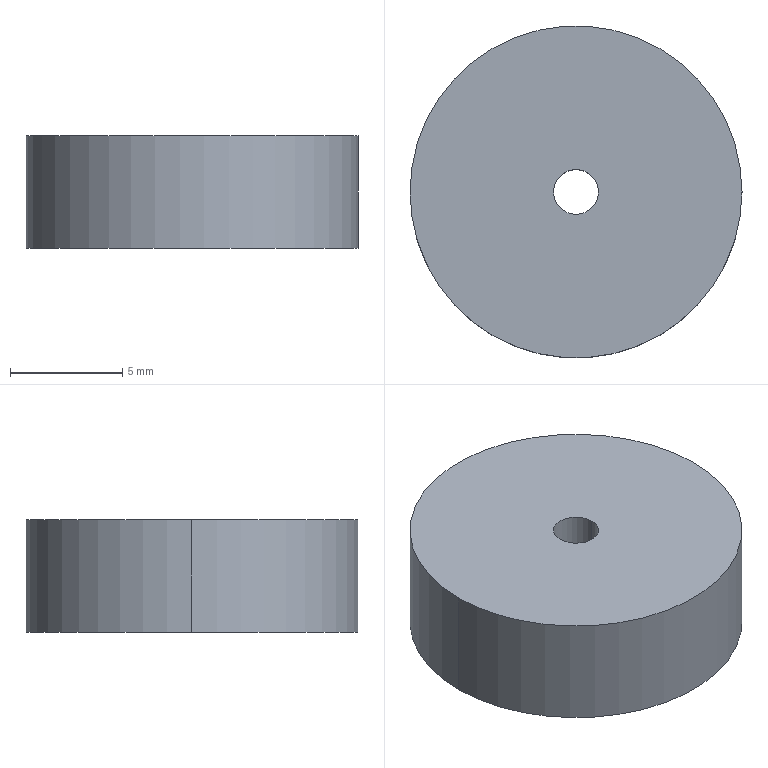Part | SolidWorks | features Extrusion 1 | 1 solid | 6 faces | box 14.8 x 14.8 x 5 mm | volume 844.46 mm3 | cylinder 4 | plane 2 | commonest cylinder face diameters 2 x2 14.8 x2
STEP:
#1=CARTESIAN_POINT('',(-1.,0.,5.));
#2=VERTEX_POINT('',#1);
#3=CARTESIAN_POINT('',(1.,0.,5.));
#4=VERTEX_POINT('',#3);
#5=CARTESIAN_POINT('',(0.,0.,5.));
#6=DIRECTION('',(0.,0.,1.));
#7=DIRECTION('',(1.,0.,0.));
#8=AXIS2_PLACEMENT_3D('',#5,#6,#7);
#9=CIRCLE('',#8,1.);
#10=EDGE_CURVE('',#2,#4,#9,.T.);
#11=ORIENTED_EDGE('',*,*,#10,.T.);
#12=CARTESIAN_POINT('',(1.,0.,0.));
#13=VERTEX_POINT('',#12);
#14=CARTESIAN_POINT('',(1.,0.,5.));
#15=DIRECTION('',(0.,0.,-1.));
#16=VECTOR('',#15,1000.);
#17=LINE('',#14,#16);
#18=EDGE_CURVE('',#4,#13,#17,.T.);
#19=ORIENTED_EDGE('',*,*,#18,.T.);
#20=CARTESIAN_POINT('',(-1.,0.,0.));
#21=VERTEX_POINT('',#20);
#22=CARTESIAN_POINT('',(0.,0.,0.));
#23=DIRECTION('',(0.,0.,1.));
#24=DIRECTION('',(1.,0.,0.));
#25=AXIS2_PLACEMENT_3D('',#22,#23,#24);
#26=CIRCLE('',#25,1.);
#27=EDGE_CURVE('',#21,#13,#26,.T.);
#28=ORIENTED_EDGE('',*,*,#27,.F.);
#29=CARTESIAN_POINT('',(-1.,0.,5.));
#30=DIRECTION('',(0.,0.,-1.));
#31=VECTOR('',#30,1000.);
#32=LINE('',#29,#31);
#33=EDGE_CURVE('',#2,#21,#32,.T.);
#34=ORIENTED_EDGE('',*,*,#33,.F.);
#35=EDGE_LOOP('',(#11,#19,#28,#34));
#36=FACE_OUTER_BOUND('',#35,.T.);
#37=CARTESIAN_POINT('',(0.,0.,5.));
#38=DIRECTION('',(0.,0.,-1.));
#39=DIRECTION('',(-1.,0.,0.));
#40=AXIS2_PLACEMENT_3D('',#37,#38,#39);
#41=CYLINDRICAL_SURFACE('',#40,1.);
#42=ADVANCED_FACE('',(#36),#41,.F.);
#43=CARTESIAN_POINT('',(7.4,0.,5.));
#44=VERTEX_POINT('',#43);
#45=CARTESIAN_POINT('',(-7.4,0.,5.));
#46=VERTEX_POINT('',#45);
#47=CARTESIAN_POINT('',(0.,0.,5.));
#48=DIRECTION('',(0.,0.,1.));
#49=DIRECTION('',(1.,0.,0.));
#50=AXIS2_PLACEMENT_3D('',#47,#48,#49);
#51=CIRCLE('',#50,7.4);
#52=EDGE_CURVE('',#44,#46,#51,.T.);
#53=ORIENTED_EDGE('',*,*,#52,.F.);
#54=CARTESIAN_POINT('',(7.4,0.,0.));
#55=VERTEX_POINT('',#54);
#56=CARTESIAN_POINT('',(7.4,0.,5.));
#57=DIRECTION('',(0.,0.,-1.));
#58=VECTOR('',#57,1000.);
#59=LINE('',#56,#58);
#60=EDGE_CURVE('',#44,#55,#59,.T.);
#61=ORIENTED_EDGE('',*,*,#60,.T.);
#62=CARTESIAN_POINT('',(-7.4,0.,0.));
#63=VERTEX_POINT('',#62);
#64=CARTESIAN_POINT('',(0.,0.,0.));
#65=DIRECTION('',(0.,0.,1.));
#66=DIRECTION('',(1.,0.,0.));
#67=AXIS2_PLACEMENT_3D('',#64,#65,#66);
#68=CIRCLE('',#67,7.4);
#69=EDGE_CURVE('',#55,#63,#68,.T.);
#70=ORIENTED_EDGE('',*,*,#69,.T.);
#71=CARTESIAN_POINT('',(-7.4,0.,5.));
#72=DIRECTION('',(0.,0.,-1.));
#73=VECTOR('',#72,1000.);
#74=LINE('',#71,#73);
#75=EDGE_CURVE('',#46,#63,#74,.T.);
#76=ORIENTED_EDGE('',*,*,#75,.F.);
#77=EDGE_LOOP('',(#53,#61,#70,#76));
#78=FACE_OUTER_BOUND('',#77,.T.);
#79=CARTESIAN_POINT('',(0.,0.,5.));
#80=DIRECTION('',(0.,0.,-1.));
#81=DIRECTION('',(-1.,0.,0.));
#82=AXIS2_PLACEMENT_3D('',#79,#80,#81);
#83=CYLINDRICAL_SURFACE('',#82,7.4);
#84=ADVANCED_FACE('',(#78),#83,.T.);
#85=CARTESIAN_POINT('',(0.,0.,5.));
#86=DIRECTION('',(0.,0.,1.));
#87=DIRECTION('',(1.,0.,0.));
#88=AXIS2_PLACEMENT_3D('',#85,#86,#87);
#89=CIRCLE('',#88,7.4);
#90=EDGE_CURVE('',#46,#44,#89,.T.);
#91=ORIENTED_EDGE('',*,*,#90,.T.);
#92=ORIENTED_EDGE('',*,*,#52,.T.);
#93=EDGE_LOOP('',(#91,#92));
#94=FACE_OUTER_BOUND('',#93,.T.);
#95=ORIENTED_EDGE('',*,*,#10,.F.);
#96=CARTESIAN_POINT('',(0.,0.,5.));
#97=DIRECTION('',(0.,0.,1.));
#98=DIRECTION('',(1.,0.,0.));
#99=AXIS2_PLACEMENT_3D('',#96,#97,#98);
#100=CIRCLE('',#99,1.);
#101=EDGE_CURVE('',#4,#2,#100,.T.);
#102=ORIENTED_EDGE('',*,*,#101,.F.);
#103=EDGE_LOOP('',(#95,#102));
#104=FACE_BOUND('',#103,.T.);
#105=CARTESIAN_POINT('',(0.,0.,5.));
#106=DIRECTION('',(0.,0.,1.));
#107=DIRECTION('',(1.,0.,0.));
#108=AXIS2_PLACEMENT_3D('',#105,#106,#107);
#109=PLANE('',#108);
#110=ADVANCED_FACE('',(#94,#104),#109,.T.);
#111=CARTESIAN_POINT('',(0.,0.,0.));
#112=DIRECTION('',(0.,0.,1.));
#113=DIRECTION('',(1.,0.,0.));
#114=AXIS2_PLACEMENT_3D('',#111,#112,#113);
#115=CIRCLE('',#114,7.4);
#116=EDGE_CURVE('',#63,#55,#115,.T.);
#117=ORIENTED_EDGE('',*,*,#116,.F.);
#118=ORIENTED_EDGE('',*,*,#69,.F.);
#119=EDGE_LOOP('',(#117,#118));
#120=FACE_OUTER_BOUND('',#119,.T.);
#121=ORIENTED_EDGE('',*,*,#27,.T.);
#122=CARTESIAN_POINT('',(0.,0.,0.));
#123=DIRECTION('',(0.,0.,1.));
#124=DIRECTION('',(1.,0.,0.));
#125=AXIS2_PLACEMENT_3D('',#122,#123,#124);
#126=CIRCLE('',#125,1.);
#127=EDGE_CURVE('',#13,#21,#126,.T.);
#128=ORIENTED_EDGE('',*,*,#127,.T.);
#129=EDGE_LOOP('',(#121,#128));
#130=FACE_BOUND('',#129,.T.);
#131=CARTESIAN_POINT('',(0.,0.,0.));
#132=DIRECTION('',(0.,0.,1.));
#133=DIRECTION('',(1.,0.,0.));
#134=AXIS2_PLACEMENT_3D('',#131,#132,#133);
#135=PLANE('',#134);
#136=ADVANCED_FACE('',(#120,#130),#135,.F.);
#137=ORIENTED_EDGE('',*,*,#60,.F.);
#138=ORIENTED_EDGE('',*,*,#90,.F.);
#139=ORIENTED_EDGE('',*,*,#75,.T.);
#140=ORIENTED_EDGE('',*,*,#116,.T.);
#141=EDGE_LOOP('',(#137,#138,#139,#140));
#142=FACE_OUTER_BOUND('',#141,.T.);
#143=CARTESIAN_POINT('',(0.,0.,5.));
#144=DIRECTION('',(0.,0.,-1.));
#145=DIRECTION('',(-1.,0.,0.));
#146=AXIS2_PLACEMENT_3D('',#143,#144,#145);
#147=CYLINDRICAL_SURFACE('',#146,7.4);
#148=ADVANCED_FACE('',(#142),#147,.T.);
#149=ORIENTED_EDGE('',*,*,#18,.F.);
#150=ORIENTED_EDGE('',*,*,#101,.T.);
#151=ORIENTED_EDGE('',*,*,#33,.T.);
#152=ORIENTED_EDGE('',*,*,#127,.F.);
#153=EDGE_LOOP('',(#149,#150,#151,#152));
#154=FACE_OUTER_BOUND('',#153,.T.);
#155=CARTESIAN_POINT('',(0.,0.,5.));
#156=DIRECTION('',(0.,0.,-1.));
#157=DIRECTION('',(-1.,0.,0.));
#158=AXIS2_PLACEMENT_3D('',#155,#156,#157);
#159=CYLINDRICAL_SURFACE('',#158,1.);
#160=ADVANCED_FACE('',(#154),#159,.F.);
#161=CLOSED_SHELL('',(#42,#84,#110,#136,#148,#160));
#162=MANIFOLD_SOLID_BREP('',#161);
#163=CARTESIAN_POINT('',(0.,0.,0.));
#164=DIRECTION('',(0.,0.,1.));
#165=DIRECTION('',(1.,0.,0.));
#166=AXIS2_PLACEMENT_3D('',#163,#164,#165);
#167=(LENGTH_UNIT()NAMED_UNIT(*)SI_UNIT(.MILLI.,.METRE.));
#168=UNCERTAINTY_MEASURE_WITH_UNIT(LENGTH_MEASURE(0.00001),#167,'','');
#169=(NAMED_UNIT(*)PLANE_ANGLE_UNIT()SI_UNIT($,.RADIAN.));
#170=(NAMED_UNIT(*)SI_UNIT($,.STERADIAN.)SOLID_ANGLE_UNIT());
#171=(GEOMETRIC_REPRESENTATION_CONTEXT(3)GLOBAL_UNCERTAINTY_ASSIGNED_CONTEXT((#168))GLOBAL_UNIT_ASSIGNED_CONTEXT((#167,#169,#170))REPRESENTATION_CONTEXT('',''));
#172=ADVANCED_BREP_SHAPE_REPRESENTATION('',(#162,#166),#171);